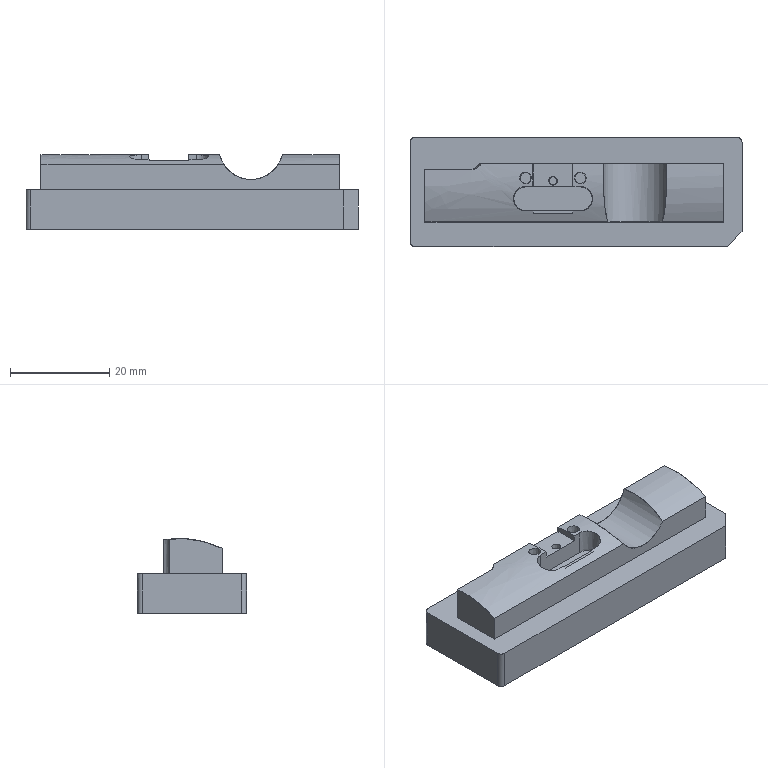NC program | PowerMill | posted with a generic post | part box 67 x 22 x 15.086 mm
Lines 17666 to 18440 of 221347:
N17763 M6
N17764 S22000 M03
N17765 G00 G90 X0.0 Y0.0
N17766 G43 Z9.7955 H27
N17767
N17768 G05 P10000 R4
N17769 X-4.5617 Y1.9439
N17770 Z-0.2426
N17771 G01 Z-1.4426 F1200.0
N17772 X-4.5093 Y1.9588 Z-1.4435
N17773 X-4.4875 Y1.965 Z-1.4439
N17774 X-4.3955 Y2.0345 Z-1.4459
N17775 X-4.3343 Y2.1329 Z-1.448
N17776 X-4.3126 Y2.2474 Z-1.45
N17777 X-4.3339 Y2.3611 Z-1.452
N17778 X-4.3945 Y2.4592 Z-1.454
N17779 X-4.441 Y2.4946 Z-1.4551
N17780 X-4.4875 Y2.5298 Z-1.4561
N17781 X-4.5983 Y2.5614 Z-1.4581
N17782 X-4.7137 Y2.5509 Z-1.4601
N17783 X-4.8179 Y2.4993 Z-1.4621
N17784 X-4.8959 Y2.4139 Z-1.4642
N17785 X-4.9382 Y2.3054 Z-1.4662
N17786 Y2.1897 Z-1.4682
N17787 X-4.8965 Y2.0817 Z-1.4702
N17788 X-4.8632 Y2.0451 Z-1.4711
N17789 X-4.8137 Y1.9937 Z-1.4723
N17790 X-4.7145 Y1.944 Z-1.4743
N17791 X-4.599 Y1.9333 Z-1.4763
N17792 X-4.5954 Y1.9343 Z-1.4764
N17793 X-4.5093 Y1.9588 Z-1.4779
N17794 X-4.4875 Y1.965 Z-1.4783
N17795 X-4.3955 Y2.0345 Z-1.4803
N17796 X-4.3343 Y2.1329 Z-1.4824
N17797 X-4.3126 Y2.2474 Z-1.4844
N17798 X-4.3339 Y2.3611 Z-1.4864
N17799 X-4.3945 Y2.4592 Z-1.4884
N17800 X-4.441 Y2.4946 Z-1.4894
N17801 X-4.4875 Y2.5298 Z-1.4905
N17802 X-4.5983 Y2.5614 Z-1.4925
N17803 X-4.7137 Y2.5509 Z-1.4945
N17804 X-4.8179 Y2.4993 Z-1.4965
N17805 X-4.8959 Y2.4139 Z-1.4985
N17806 X-4.9382 Y2.3054 Z-1.5006
N17807 Y2.1897 Z-1.5026
N17808 X-4.8965 Y2.0817 Z-1.5046
N17809 X-4.8632 Y2.0451 Z-1.5055
N17810 X-4.8137 Y1.9937 Z-1.5067
N17811 X-4.7145 Y1.944 Z-1.5087
N17812 X-4.599 Y1.9333 Z-1.5107
N17813 X-4.5954 Y1.9343
N17814 X-4.5093 Y1.9588 Z-1.5123
N17815 X-4.4875 Y1.965 Z-1.5127
N17816 X-4.3955 Y2.0345 Z-1.5147
N17817 X-4.3343 Y2.1329 Z-1.5167
N17818 X-4.3126 Y2.2474 Z-1.5188
N17819 X-4.3339 Y2.3611 Z-1.5208
N17820 X-4.3945 Y2.4592 Z-1.5228
N17821 X-4.441 Y2.4946 Z-1.5238
N17822 X-4.4875 Y2.5298 Z-1.5248
N17823 X-4.5983 Y2.5614 Z-1.5269
N17824 X-4.7137 Y2.5509 Z-1.5289
N17825 X-4.8179 Y2.4993 Z-1.5309
N17826 X-4.8959 Y2.4139 Z-1.5329
N17827 X-4.9382 Y2.3054 Z-1.535
N17828 Y2.1897 Z-1.537
N17829 X-4.8965 Y2.0817 Z-1.539
N17830 X-4.8632 Y2.0451 Z-1.5399
N17831 X-4.8137 Y1.9937 Z-1.5411
N17832 X-4.7145 Y1.944 Z-1.543
N17833 X-4.599 Y1.9333 Z-1.5451
N17834 X-4.5954 Y1.9343
N17835 X-4.5093 Y1.9588 Z-1.5467
N17836 X-4.4875 Y1.965 Z-1.5471
N17837 X-4.3955 Y2.0345 Z-1.5491
N17838 X-4.3343 Y2.1329 Z-1.5511
N17839 X-4.3126 Y2.2474 Z-1.5532
N17840 X-4.3339 Y2.3611 Z-1.5552
N17841 X-4.3945 Y2.4592 Z-1.5572
N17842 X-4.441 Y2.4946 Z-1.5582
N17843 X-4.4875 Y2.5298 Z-1.5592
N17844 X-4.5983 Y2.5614 Z-1.5612
N17845 X-4.7137 Y2.5509 Z-1.5633
N17846 X-4.8179 Y2.4993 Z-1.5653
N17847 X-4.8959 Y2.4139 Z-1.5673
N17848 X-4.9382 Y2.3054 Z-1.5693
N17849 Y2.1897 Z-1.5714
N17850 X-4.8965 Y2.0817 Z-1.5734
N17851 X-4.8632 Y2.0451 Z-1.5742
N17852 X-4.8137 Y1.9937 Z-1.5755
N17853 X-4.7145 Y1.944 Z-1.5774
N17854 X-4.599 Y1.9333 Z-1.5794
N17855 X-4.5954 Y1.9343 Z-1.5795
N17856 X-4.5093 Y1.9588 Z-1.5811
N17857 X-4.4875 Y1.965 Z-1.5815
N17858 X-4.3955 Y2.0345 Z-1.5835
N17859 X-4.3343 Y2.1329 Z-1.5855
N17860 X-4.3126 Y2.2474 Z-1.5875
N17861 X-4.3339 Y2.3611 Z-1.5896
N17862 X-4.3945 Y2.4592 Z-1.5916
N17863 X-4.441 Y2.4946 Z-1.5926
N17864 X-4.4229 Y2.5184
N17865 X-4.4739 Y2.5572 F2000.0
N17866 X-4.5955 Y2.5918
N17867 X-4.722 Y2.5803
N17868 X-4.8363 Y2.5237
N17869 X-4.9219 Y2.43
N17870 X-4.9682 Y2.311
N17871 Y2.1841
N17872 X-4.9224 Y2.0656
N17873 X-4.8851 Y2.0246
N17874 X-4.8317 Y1.9692
N17875 X-4.7229 Y1.9147
N17876 X-4.5962 Y1.9029
N17877 X-4.5872 Y1.9055
N17878 X-4.5011 Y1.93
N17879 X-4.4739 Y1.9377
N17880 X-4.3729 Y2.0139
N17881 X-4.3058 Y2.1218
N17882 X-4.2821 Y2.2473
N17883 X-4.3054 Y2.3722
N17884 X-4.3719 Y2.4797
N17885 X-4.4229 Y2.5184
N17886 X-4.5844 Y1.9385 Z-1.4919
N17887 X-4.5123 Y1.9588 Z-1.4932 F1200.0
N17888 X-4.488 Y1.9657 Z-1.4937
N17889 X-4.3961 Y2.0351 Z-1.4957
N17890 X-4.335 Y2.1333 Z-1.4977
N17891 X-4.3136 Y2.247 Z-1.4997
N17892 X-4.3347 Y2.3607 Z-1.5017
N17893 X-4.3951 Y2.4587 Z-1.5037
N17894 X-4.4415 Y2.4939 Z-1.5048
N17895 X-4.4873 Y2.5286 Z-1.5058
N17896 X-4.5989 Y2.5607 Z-1.5078
N17897 X-4.7137 Y2.5501 Z-1.5098
N17898 X-4.8174 Y2.4986 Z-1.5118
N17899 X-4.8954 Y2.4132 Z-1.5138
N17900 X-4.9372 Y2.3056 Z-1.5159
N17901 X-4.9374 Y2.1904 Z-1.5179
N17902 X-4.8959 Y2.0826 Z-1.5199
N17903 X-4.84 Y2.021 Z-1.5213
N17904 X-4.815 Y1.995 Z-1.522
N17905 X-4.7147 Y1.9451 Z-1.5239
N17906 X-4.5996 Y1.9342 Z-1.5259
N17907 X-4.596 Y1.9352 Z-1.526
N17908 X-4.5123 Y1.9588 Z-1.5275
N17909 X-4.488 Y1.9657 Z-1.528
N17910 X-4.3961 Y2.0351 Z-1.53
N17911 X-4.335 Y2.1333 Z-1.532
N17912 X-4.3136 Y2.247 Z-1.534
N17913 X-4.3347 Y2.3607 Z-1.536
N17914 X-4.3951 Y2.4587 Z-1.538
N17915 X-4.4415 Y2.4939 Z-1.539
N17916 X-4.4873 Y2.5286 Z-1.5401
N17917 X-4.5989 Y2.5607 Z-1.5421
N17918 X-4.7137 Y2.5501 Z-1.5441
N17919 X-4.8174 Y2.4986 Z-1.5461
N17920 X-4.8954 Y2.4132 Z-1.5481
N17921 X-4.9372 Y2.3056 Z-1.5501
N17922 X-4.9374 Y2.1904 Z-1.5522
N17923 X-4.8959 Y2.0826 Z-1.5542
N17924 X-4.84 Y2.021 Z-1.5556
N17925 X-4.815 Y1.995 Z-1.5563
N17926 X-4.7147 Y1.9451 Z-1.5582
N17927 X-4.5996 Y1.9342 Z-1.5602
N17928 X-4.596 Y1.9352 Z-1.5603
N17929 X-4.5123 Y1.9588 Z-1.5618
N17930 X-4.488 Y1.9657 Z-1.5622
N17931 X-4.3961 Y2.0351 Z-1.5643
N17932 X-4.335 Y2.1333 Z-1.5663
N17933 X-4.3136 Y2.247 Z-1.5683
N17934 X-4.3347 Y2.3607 Z-1.5703
N17935 X-4.3951 Y2.4587 Z-1.5723
N17936 X-4.4415 Y2.4939 Z-1.5733
N17937 X-4.4873 Y2.5286 Z-1.5743
N17938 X-4.5989 Y2.5607 Z-1.5764
N17939 X-4.7137 Y2.5501 Z-1.5784
N17940 X-4.8174 Y2.4986 Z-1.5804
N17941 X-4.8954 Y2.4132 Z-1.5824
N17942 X-4.9372 Y2.3056 Z-1.5844
N17943 X-4.9374 Y2.1904 Z-1.5864
N17944 X-4.8959 Y2.0826 Z-1.5885
N17945 X-4.84 Y2.021 Z-1.5899
N17946 X-4.815 Y1.995 Z-1.5905
N17947 X-4.7147 Y1.9451 Z-1.5925
N17948 X-4.5996 Y1.9342 Z-1.5945
N17949 X-4.596 Y1.9352 Z-1.5946
N17950 X-4.5123 Y1.9588 Z-1.5961
N17951 X-4.488 Y1.9657 Z-1.5965
N17952 X-4.3961 Y2.0351 Z-1.5985
N17953 X-4.335 Y2.1333 Z-1.6006
N17954 X-4.3136 Y2.247 Z-1.6026
N17955 X-4.3347 Y2.3607 Z-1.6046
N17956 X-4.3951 Y2.4587 Z-1.6066
N17957 X-4.4415 Y2.4939 Z-1.6076
N17958 X-4.4873 Y2.5286 Z-1.6086
N17959 X-4.5989 Y2.5607 Z-1.6107
N17960 X-4.7137 Y2.5501 Z-1.6127
N17961 X-4.8174 Y2.4986 Z-1.6147
N17962 X-4.8954 Y2.4132 Z-1.6167
N17963 X-4.9372 Y2.3056 Z-1.6187
N17964 X-4.9374 Y2.1904 Z-1.6207
N17965 X-4.8959 Y2.0826 Z-1.6228
N17966 X-4.84 Y2.021 Z-1.6242
N17967 X-4.815 Y1.995 Z-1.6248
N17968 X-4.7147 Y1.9451 Z-1.6268
N17969 X-4.5996 Y1.9342 Z-1.6288
N17970 X-4.596 Y1.9352 Z-1.6289
N17971 X-4.5123 Y1.9588 Z-1.6304
N17972 X-4.488 Y1.9657 Z-1.6308
N17973 X-4.3961 Y2.0351 Z-1.6328
N17974 X-4.335 Y2.1333 Z-1.6349
N17975 X-4.3136 Y2.247 Z-1.6369
N17976 X-4.3347 Y2.3607 Z-1.6389
N17977 X-4.3951 Y2.4587 Z-1.6409
N17978 X-4.4415 Y2.4939 Z-1.6419
N17979 X-4.4234 Y2.5178
N17980 X-4.4736 Y2.5559 F2000.0
N17981 X-4.596 Y2.591
N17982 X-4.722 Y2.5794
N17983 X-4.8358 Y2.523
N17984 X-4.9214 Y2.4293
N17985 X-4.9672 Y2.3112
N17986 X-4.9674 Y2.1849
N17987 X-4.9219 Y2.0666
N17988 X-4.8619 Y2.0005
N17989 X-4.833 Y1.9705
N17990 X-4.7231 Y1.9157
N17991 X-4.5968 Y1.9038
N17992 X-4.5878 Y1.9063
N17993 X-4.5041 Y1.93
N17994 X-4.4744 Y1.9384
N17995 X-4.3736 Y2.0145
N17996 X-4.3066 Y2.1223
N17997 X-4.283 Y2.247
N17998 X-4.3062 Y2.3717
N17999 X-4.3726 Y2.4792
N18000 X-4.4234 Y2.5178
N18001 X-4.6067 Y1.9357 Z-1.5412
N18002 X-4.5996 Y1.935 Z-1.5414 F1200.0
N18003 X-4.596 Y1.936
N18004 X-4.5154 Y1.9588 Z-1.5429
N18005 X-4.4889 Y1.9664 Z-1.5434
N18006 X-4.3968 Y2.0356 Z-1.5454
N18007 X-4.3359 Y2.1335 Z-1.5474
N18008 X-4.3144 Y2.2473 Z-1.5494
N18009 X-4.3354 Y2.36 Z-1.5514
N18010 X-4.3962 Y2.4588 Z-1.5535
N18011 X-4.4419 Y2.4933 Z-1.5545
N18012 X-4.4876 Y2.5278 Z-1.5555
N18013 X-4.5988 Y2.5597 Z-1.5575
N18014 X-4.7132 Y2.5493 Z-1.5595
N18015 X-4.8172 Y2.4978 Z-1.5615
N18016 X-4.8948 Y2.4127 Z-1.5635
N18017 X-4.9364 Y2.3055 Z-1.5655
N18018 X-4.9365 Y2.1903 Z-1.5675
N18019 X-4.8951 Y2.0829 Z-1.5695
N18020 X-4.8198 Y1.9999 Z-1.5715
N18021 X-4.8171 Y1.9971 Z-1.5716
N18022 X-4.714 Y1.9457 Z-1.5736
N18023 X-4.5996 Y1.935 Z-1.5756
N18024 X-4.596 Y1.936
N18025 X-4.5154 Y1.9588 Z-1.5771
N18026 X-4.4889 Y1.9664 Z-1.5776
N18027 X-4.3968 Y2.0356 Z-1.5796
N18028 X-4.3359 Y2.1335 Z-1.5816
N18029 X-4.3144 Y2.2473 Z-1.5836
N18030 X-4.3354 Y2.36 Z-1.5856
N18031 X-4.3962 Y2.4588 Z-1.5877
N18032 X-4.4419 Y2.4933 Z-1.5887
N18033 X-4.4876 Y2.5278 Z-1.5897
N18034 X-4.5988 Y2.5597 Z-1.5917
N18035 X-4.7132 Y2.5493 Z-1.5937
N18036 X-4.8172 Y2.4978 Z-1.5957
N18037 X-4.8948 Y2.4127 Z-1.5977
N18038 X-4.9364 Y2.3055 Z-1.5997
N18039 X-4.9365 Y2.1903 Z-1.6017
N18040 X-4.8951 Y2.0829 Z-1.6037
N18041 X-4.8198 Y1.9999 Z-1.6057
N18042 X-4.8171 Y1.9971 Z-1.6058
N18043 X-4.714 Y1.9457 Z-1.6078
N18044 X-4.5996 Y1.935 Z-1.6098
N18045 X-4.596 Y1.936
N18046 X-4.5154 Y1.9588 Z-1.6113
N18047 X-4.4889 Y1.9664 Z-1.6118
N18048 X-4.3968 Y2.0356 Z-1.6138
N18049 X-4.3359 Y2.1335 Z-1.6158
N18050 X-4.3144 Y2.2473 Z-1.6178
N18051 X-4.3354 Y2.36 Z-1.6198
N18052 X-4.3962 Y2.4588 Z-1.6219
N18053 X-4.4419 Y2.4933 Z-1.6229
N18054 X-4.4876 Y2.5278 Z-1.6239
N18055 X-4.5988 Y2.5597 Z-1.6259
N18056 X-4.7132 Y2.5493 Z-1.6279
N18057 X-4.8172 Y2.4978 Z-1.6299
N18058 X-4.8948 Y2.4127 Z-1.6319
N18059 X-4.9364 Y2.3055 Z-1.6339
N18060 X-4.9365 Y2.1903 Z-1.6359
N18061 X-4.8951 Y2.0829 Z-1.6379
N18062 X-4.8198 Y1.9999 Z-1.6399
N18063 X-4.8171 Y1.9971 Z-1.64
N18064 X-4.714 Y1.9457 Z-1.642
N18065 X-4.5996 Y1.935 Z-1.644
N18066 X-4.596 Y1.936
N18067 X-4.5154 Y1.9588 Z-1.6455
N18068 X-4.4889 Y1.9664 Z-1.646
N18069 X-4.3968 Y2.0356 Z-1.648
N18070 X-4.3359 Y2.1335 Z-1.65
N18071 X-4.3144 Y2.2473 Z-1.652
N18072 X-4.3354 Y2.36 Z-1.654
N18073 X-4.3962 Y2.4588 Z-1.6561
N18074 X-4.4419 Y2.4933 Z-1.6571
N18075 X-4.4876 Y2.5278 Z-1.6581
N18076 X-4.5988 Y2.5597 Z-1.6601
N18077 X-4.7132 Y2.5493 Z-1.6621
N18078 X-4.8172 Y2.4978 Z-1.6641
N18079 X-4.8948 Y2.4127 Z-1.6661
N18080 X-4.9364 Y2.3055 Z-1.6681
N18081 X-4.9365 Y2.1903 Z-1.6701
N18082 X-4.8951 Y2.0829 Z-1.6721
N18083 X-4.8198 Y1.9999 Z-1.6741
N18084 X-4.8171 Y1.9971 Z-1.6742
N18085 X-4.714 Y1.9457 Z-1.6762
N18086 X-4.5996 Y1.935 Z-1.6782
N18087 X-4.596 Y1.936
N18088 X-4.5154 Y1.9588 Z-1.6797
N18089 X-4.4889 Y1.9664 Z-1.6802
N18090 X-4.3968 Y2.0356 Z-1.6822
N18091 X-4.3359 Y2.1335 Z-1.6842
N18092 X-4.3144 Y2.2473 Z-1.6862
N18093 X-4.3354 Y2.36 Z-1.6882
N18094 X-4.3962 Y2.4588 Z-1.6903
N18095 X-4.4419 Y2.4933 Z-1.6912
N18096 X-4.4238 Y2.5172
N18097 X-4.474 Y2.5551 F2000.0
N18098 X-4.5959 Y2.5901
N18099 X-4.7215 Y2.5786
N18100 X-4.8355 Y2.5222
N18101 X-4.9207 Y2.4288
N18102 X-4.9663 Y2.3112
N18103 X-4.9665 Y2.1847
N18104 X-4.9211 Y2.0669
N18105 X-4.8417 Y1.9795
N18106 X-4.8351 Y1.9726
N18107 X-4.7224 Y1.9163
N18108 X-4.5968 Y1.9046
N18109 X-4.5879 Y1.9072
N18110 X-4.5072 Y1.93
N18111 X-4.4753 Y1.939
N18112 X-4.3743 Y2.015
N18113 X-4.3075 Y2.1224
N18114 X-4.2839 Y2.2472
N18115 X-4.3069 Y2.371
N18116 X-4.3736 Y2.4793
N18117 X-4.4238 Y2.5172
N18118 X-4.6301 Y1.9387 Z-1.5906
N18119 X-4.5996 Y1.9359 Z-1.5911 F1200.0
N18120 X-4.596 Y1.9369 Z-1.5912
N18121 X-4.5185 Y1.9588 Z-1.5926
N18122 X-4.4889 Y1.9672 Z-1.5931
N18123 X-4.3972 Y2.0364 Z-1.5951
N18124 X-4.3365 Y2.1341 Z-1.5971
N18125 X-4.3153 Y2.2471 Z-1.5991
N18126 X-4.3362 Y2.3599 Z-1.6011
N18127 X-4.3966 Y2.4578 Z-1.6031
N18128 X-4.4425 Y2.4926 Z-1.6041
N18129 X-4.4879 Y2.527 Z-1.6051
N18130 X-4.5986 Y2.5588 Z-1.6072
N18131 X-4.7129 Y2.5485 Z-1.6092
N18132 X-4.8163 Y2.4973 Z-1.6112
N18133 X-4.894 Y2.4124 Z-1.6132
N18134 X-4.9356 Y2.3051 Z-1.6152
N18135 X-4.9357 Y2.1901 Z-1.6172
N18136 X-4.8945 Y2.0836 Z-1.6192
N18137 X-4.8171 Y1.9982 Z-1.6212
N18138 X-4.7139 Y1.9466 Z-1.6232
N18139 X-4.5996 Y1.9359 Z-1.6252
N18140 X-4.596 Y1.9369 Z-1.6253
N18141 X-4.5185 Y1.9588 Z-1.6267
N18142 X-4.4889 Y1.9672 Z-1.6272
N18143 X-4.3972 Y2.0364 Z-1.6292
N18144 X-4.3365 Y2.1341 Z-1.6312
N18145 X-4.3153 Y2.2471 Z-1.6332
N18146 X-4.3362 Y2.3599 Z-1.6352
N18147 X-4.3966 Y2.4578 Z-1.6372
N18148 X-4.4425 Y2.4926 Z-1.6383
N18149 X-4.4879 Y2.527 Z-1.6392
N18150 X-4.5986 Y2.5588 Z-1.6413
N18151 X-4.7129 Y2.5485 Z-1.6433
N18152 X-4.8163 Y2.4973 Z-1.6453
N18153 X-4.894 Y2.4124 Z-1.6473
N18154 X-4.9356 Y2.3051 Z-1.6493
N18155 X-4.9357 Y2.1901 Z-1.6513
N18156 X-4.8945 Y2.0836 Z-1.6533
N18157 X-4.8171 Y1.9982 Z-1.6553
N18158 X-4.7139 Y1.9466 Z-1.6573
N18159 X-4.5996 Y1.9359 Z-1.6593
N18160 X-4.596 Y1.9369 Z-1.6594
N18161 X-4.5185 Y1.9588 Z-1.6608
N18162 X-4.4889 Y1.9672 Z-1.6613
N18163 X-4.3972 Y2.0364 Z-1.6633
N18164 X-4.3365 Y2.1341 Z-1.6653
N18165 X-4.3153 Y2.2471 Z-1.6673
N18166 X-4.3362 Y2.3599 Z-1.6693
N18167 X-4.3966 Y2.4578 Z-1.6714
N18168 X-4.4425 Y2.4926 Z-1.6724
N18169 X-4.4879 Y2.527 Z-1.6734
N18170 X-4.5986 Y2.5588 Z-1.6754
N18171 X-4.7129 Y2.5485 Z-1.6774
N18172 X-4.8163 Y2.4973 Z-1.6794
N18173 X-4.894 Y2.4124 Z-1.6814
N18174 X-4.9356 Y2.3051 Z-1.6834
N18175 X-4.9357 Y2.1901 Z-1.6854
N18176 X-4.8945 Y2.0836 Z-1.6874
N18177 X-4.8171 Y1.9982 Z-1.6894
N18178 X-4.7139 Y1.9466 Z-1.6914
N18179 X-4.5996 Y1.9359 Z-1.6934
N18180 X-4.596 Y1.9369 Z-1.6935
N18181 X-4.5185 Y1.9588 Z-1.6949
N18182 X-4.4889 Y1.9672 Z-1.6954
N18183 X-4.3972 Y2.0364 Z-1.6974
N18184 X-4.3365 Y2.1341 Z-1.6994
N18185 X-4.3153 Y2.2471 Z-1.7014
N18186 X-4.3362 Y2.3599 Z-1.7035
N18187 X-4.3966 Y2.4578 Z-1.7055
N18188 X-4.4425 Y2.4926 Z-1.7065
N18189 X-4.4879 Y2.527 Z-1.7075
N18190 X-4.5986 Y2.5588 Z-1.7095
N18191 X-4.7129 Y2.5485 Z-1.7115
N18192 X-4.8163 Y2.4973 Z-1.7135
N18193 X-4.894 Y2.4124 Z-1.7155
N18194 X-4.9356 Y2.3051 Z-1.7175
N18195 X-4.9357 Y2.1901 Z-1.7195
N18196 X-4.8945 Y2.0836 Z-1.7215
N18197 X-4.8171 Y1.9982 Z-1.7235
N18198 X-4.7139 Y1.9466 Z-1.7255
N18199 X-4.5996 Y1.9359 Z-1.7275
N18200 X-4.596 Y1.9369 Z-1.7276
N18201 X-4.5185 Y1.9588 Z-1.729
N18202 X-4.4889 Y1.9672 Z-1.7295
N18203 X-4.3972 Y2.0364 Z-1.7315
N18204 X-4.3365 Y2.1341 Z-1.7335
N18205 X-4.3153 Y2.2471 Z-1.7356
N18206 X-4.3362 Y2.3599 Z-1.7376
N18207 X-4.3966 Y2.4578 Z-1.7396
N18208 X-4.4425 Y2.4926 Z-1.7406
N18209 X-4.4244 Y2.5165
N18210 X-4.4743 Y2.5543 F2000.0
N18211 X-4.5957 Y2.5892
N18212 X-4.7212 Y2.5778
N18213 X-4.8346 Y2.5217
N18214 X-4.9199 Y2.4284
N18215 X-4.9656 Y2.3107
N18216 X-4.9657 Y2.1845
N18217 X-4.9204 Y2.0675
N18218 X-4.8356 Y1.9739
N18219 X-4.7223 Y1.9172
N18220 X-4.5968 Y1.9055
N18221 X-4.5879 Y1.908
N18222 X-4.5103 Y1.93
N18223 X-4.4754 Y1.9399
N18224 X-4.3746 Y2.0158
N18225 X-4.3081 Y2.123
N18226 X-4.2847 Y2.247
N18227 X-4.3078 Y2.3709
N18228 X-4.374 Y2.4784
N18229 X-4.4244 Y2.5165
N18230 X-4.6814 Y1.9444 Z-1.6399
N18231 X-4.5996 Y1.9367 Z-1.6413 F1200.0
N18232 X-4.5216 Y1.9588 Z-1.6427
N18233 X-4.4897 Y1.9679 Z-1.6433
N18234 X-4.4044 Y2.032 Z-1.6452
N18235 X-4.3978 Y2.0408 Z-1.6454
N18236 X-4.3188 Y2.2442 Z-1.6492
N18237 X-4.3178 Y2.2551 Z-1.6494
N18238 X-4.337 Y2.3596 Z-1.6512
N18239 X-4.3971 Y2.457 Z-1.6532
N18240 X-4.443 Y2.4919 Z-1.6542
N18241 X-4.4883 Y2.5262 Z-1.6552
N18242 X-4.5993 Y2.5581 Z-1.6572
N18243 X-4.7132 Y2.5476 Z-1.6592
N18244 X-4.8157 Y2.4967 Z-1.6612
N18245 X-4.8934 Y2.4117 Z-1.6632
N18246 X-4.9346 Y2.3053 Z-1.6652
N18247 X-4.9348 Y2.1906 Z-1.6672
N18248 X-4.8935 Y2.0835 Z-1.6692
N18249 X-4.8163 Y1.9986 Z-1.6712
N18250 X-4.7137 Y1.9474 Z-1.6732
N18251 X-4.5996 Y1.9367 Z-1.6752
N18252 X-4.5216 Y1.9588 Z-1.6767
N18253 X-4.4897 Y1.9679 Z-1.6772
N18254 X-4.4044 Y2.032 Z-1.6791
N18255 X-4.3978 Y2.0408 Z-1.6793
N18256 X-4.3188 Y2.2442 Z-1.6831
N18257 X-4.3178 Y2.2551 Z-1.6833
N18258 X-4.337 Y2.3596 Z-1.6852
N18259 X-4.3971 Y2.457 Z-1.6871
N18260 X-4.443 Y2.4919 Z-1.6882
N18261 X-4.4883 Y2.5262 Z-1.6891
N18262 X-4.5993 Y2.5581 Z-1.6912
N18263 X-4.7132 Y2.5476 Z-1.6932
N18264 X-4.8157 Y2.4967 Z-1.6952
N18265 X-4.8934 Y2.4117 Z-1.6972
N18266 X-4.9346 Y2.3053 Z-1.6992
N18267 X-4.9348 Y2.1906 Z-1.7012
N18268 X-4.8935 Y2.0835 Z-1.7032
N18269 X-4.8163 Y1.9986 Z-1.7052
N18270 X-4.7137 Y1.9474 Z-1.7072
N18271 X-4.5996 Y1.9367 Z-1.7092
N18272 X-4.5216 Y1.9588 Z-1.7106
N18273 X-4.4897 Y1.9679 Z-1.7112
N18274 X-4.4044 Y2.032 Z-1.713
N18275 X-4.3978 Y2.0408 Z-1.7132
N18276 X-4.3188 Y2.2442 Z-1.717
N18277 X-4.3178 Y2.2551 Z-1.7172
N18278 X-4.337 Y2.3596 Z-1.7191
N18279 X-4.3971 Y2.457 Z-1.7211
N18280 X-4.443 Y2.4919 Z-1.7221
N18281 X-4.4883 Y2.5262 Z-1.7231
N18282 X-4.5993 Y2.5581 Z-1.7251
N18283 X-4.7132 Y2.5476 Z-1.7271
N18284 X-4.8157 Y2.4967 Z-1.7291
N18285 X-4.8934 Y2.4117 Z-1.7311
N18286 X-4.9346 Y2.3053 Z-1.7331
N18287 X-4.9348 Y2.1906 Z-1.7351
N18288 X-4.8935 Y2.0835 Z-1.7371
N18289 X-4.8163 Y1.9986 Z-1.7391
N18290 X-4.7137 Y1.9474 Z-1.7411
N18291 X-4.5996 Y1.9367 Z-1.7431
N18292 X-4.5216 Y1.9588 Z-1.7445
N18293 X-4.4897 Y1.9679 Z-1.7451
N18294 X-4.4044 Y2.032 Z-1.7469
N18295 X-4.3978 Y2.0408 Z-1.7471
N18296 X-4.3188 Y2.2442 Z-1.7509
N18297 X-4.3178 Y2.2551 Z-1.7511
N18298 X-4.337 Y2.3596 Z-1.753
N18299 X-4.3971 Y2.457 Z-1.755
N18300 X-4.443 Y2.4919 Z-1.756
N18301 X-4.4883 Y2.5262 Z-1.757
N18302 X-4.5993 Y2.5581 Z-1.759
N18303 X-4.7132 Y2.5476 Z-1.761
N18304 X-4.8157 Y2.4967 Z-1.763
N18305 X-4.8934 Y2.4117 Z-1.765
N18306 X-4.9346 Y2.3053 Z-1.767
N18307 X-4.9348 Y2.1906 Z-1.769
N18308 X-4.8935 Y2.0835 Z-1.771
N18309 X-4.8163 Y1.9986 Z-1.773
N18310 X-4.7137 Y1.9474 Z-1.775
N18311 X-4.5996 Y1.9367 Z-1.777
N18312 X-4.5216 Y1.9588 Z-1.7784
N18313 X-4.4897 Y1.9679 Z-1.779
N18314 X-4.4044 Y2.032 Z-1.7809
N18315 X-4.3978 Y2.0408 Z-1.781
N18316 X-4.3188 Y2.2442 Z-1.7849
N18317 X-4.3178 Y2.2551 Z-1.785
N18318 X-4.337 Y2.3596 Z-1.7869
N18319 X-4.3971 Y2.457 Z-1.7889
N18320 X-4.443 Y2.4919 Z-1.7899
N18321 X-4.4249 Y2.5158
N18322 X-4.4747 Y2.5535 F2000.0
N18323 X-4.5964 Y2.5885
N18324 X-4.7216 Y2.5769
N18325 X-4.834 Y2.5211
N18326 X-4.9193 Y2.4278
N18327 X-4.9646 Y2.3109
N18328 X-4.9648 Y2.1851
N18329 X-4.9195 Y2.0675
N18330 X-4.8347 Y1.9743
N18331 X-4.7221 Y1.9181
N18332 X-4.5968 Y1.9064
N18333 X-4.5134 Y1.93
N18334 X-4.4761 Y1.9406
N18335 X-4.3864 Y2.0081
N18336 X-4.3766 Y2.0178
N18337 X-4.3698 Y2.0299
N18338 X-4.2908 Y2.2334
N18339 X-4.2877 Y2.2468
N18340 X-4.2883 Y2.2606
N18341 X-4.3086 Y2.3706
N18342 X-4.3745 Y2.4775
N18343 X-4.4249 Y2.5158
N18344 X-4.7051 Y1.9474 Z-1.6892
N18345 X-4.5996 Y1.9376 Z-1.6911 F1200.0
N18346 X-4.5247 Y1.9588 Z-1.6924
N18347 X-4.4896 Y1.9688 Z-1.6931
N18348 X-4.4054 Y2.0323 Z-1.6949
N18349 X-4.3988 Y2.041 Z-1.6951
N18350 X-4.3196 Y2.2448 Z-1.6989
N18351 X-4.3185 Y2.2557 Z-1.6991
N18352 X-4.3378 Y2.3593 Z-1.7009
N18353 X-4.3977 Y2.4563 Z-1.7029
N18354 X-4.4436 Y2.4912 Z-1.7039
N18355 X-4.4889 Y2.5256 Z-1.7049
N18356 X-4.5991 Y2.5572 Z-1.7069
N18357 X-4.7124 Y2.5468 Z-1.7089
N18358 X-4.8156 Y2.4958 Z-1.7109
N18359 X-4.8924 Y2.4116 Z-1.7129
N18360 X-4.9337 Y2.3053 Z-1.7149
N18361 X-4.934 Y2.1904 Z-1.7169
N18362 X-4.8928 Y2.0838 Z-1.7189
N18363 X-4.8161 Y1.9996 Z-1.7209
N18364 X-4.7134 Y1.9482 Z-1.7229
N18365 X-4.5996 Y1.9376 Z-1.7249
N18366 X-4.5247 Y1.9588 Z-1.7262
N18367 X-4.4896 Y1.9688 Z-1.7269
N18368 X-4.4054 Y2.0323 Z-1.7287
N18369 X-4.3988 Y2.041 Z-1.7289
N18370 X-4.3196 Y2.2448 Z-1.7327
N18371 X-4.3185 Y2.2557 Z-1.7329
N18372 X-4.3378 Y2.3593 Z-1.7348
N18373 X-4.3977 Y2.4563 Z-1.7368
N18374 X-4.4436 Y2.4912 Z-1.7378
N18375 X-4.4889 Y2.5256 Z-1.7388
N18376 X-4.5991 Y2.5572 Z-1.7408
N18377 X-4.7124 Y2.5468 Z-1.7427
N18378 X-4.8156 Y2.4958 Z-1.7447
N18379 X-4.8924 Y2.4116 Z-1.7467
N18380 X-4.9337 Y2.3053 Z-1.7487
N18381 X-4.934 Y2.1904 Z-1.7507
N18382 X-4.8928 Y2.0838 Z-1.7527
N18383 X-4.8161 Y1.9996 Z-1.7547
N18384 X-4.7134 Y1.9482 Z-1.7567
N18385 X-4.5996 Y1.9376 Z-1.7587
N18386 X-4.5247 Y1.9588 Z-1.7601
N18387 X-4.4896 Y1.9688 Z-1.7607
N18388 X-4.4054 Y2.0323 Z-1.7625
N18389 X-4.3988 Y2.041 Z-1.7627
N18390 X-4.3196 Y2.2448 Z-1.7666
N18391 X-4.3185 Y2.2557 Z-1.7667
N18392 X-4.3378 Y2.3593 Z-1.7686
N18393 X-4.3977 Y2.4563 Z-1.7706
N18394 X-4.4436 Y2.4912 Z-1.7716
N18395 X-4.4889 Y2.5256 Z-1.7726
N18396 X-4.5991 Y2.5572 Z-1.7746
N18397 X-4.7124 Y2.5468 Z-1.7766
N18398 X-4.8156 Y2.4958 Z-1.7786
N18399 X-4.8924 Y2.4116 Z-1.7806
N18400 X-4.9337 Y2.3053 Z-1.7825
N18401 X-4.934 Y2.1904 Z-1.7846
N18402 X-4.8928 Y2.0838 Z-1.7865
N18403 X-4.8161 Y1.9996 Z-1.7885
N18404 X-4.7134 Y1.9482 Z-1.7905
N18405 X-4.5996 Y1.9376 Z-1.7925
N18406 X-4.5247 Y1.9588 Z-1.7939
N18407 X-4.4896 Y1.9688 Z-1.7945
N18408 X-4.4054 Y2.0323 Z-1.7964
N18409 X-4.3988 Y2.041 Z-1.7966
N18410 X-4.3196 Y2.2448 Z-1.8004
N18411 X-4.3185 Y2.2557 Z-1.8006
N18412 X-4.3378 Y2.3593 Z-1.8024
N18413 X-4.3977 Y2.4563 Z-1.8044
N18414 X-4.4436 Y2.4912 Z-1.8054
N18415 X-4.4889 Y2.5256 Z-1.8064
N18416 X-4.5991 Y2.5572 Z-1.8084
N18417 X-4.7124 Y2.5468 Z-1.8104
N18418 X-4.8156 Y2.4958 Z-1.8124
N18419 X-4.8924 Y2.4116 Z-1.8144
N18420 X-4.9337 Y2.3053 Z-1.8164
N18421 X-4.934 Y2.1904 Z-1.8184
N18422 X-4.8928 Y2.0838 Z-1.8204
N18423 X-4.8161 Y1.9996 Z-1.8224
N18424 X-4.7134 Y1.9482 Z-1.8244
N18425 X-4.5996 Y1.9376 Z-1.8264
N18426 X-4.5247 Y1.9588 Z-1.8277
N18427 X-4.4896 Y1.9688 Z-1.8283
N18428 X-4.4054 Y2.0323 Z-1.8302
N18429 X-4.3988 Y2.041 Z-1.8304
N18430 X-4.3196 Y2.2448 Z-1.8342
N18431 X-4.3185 Y2.2557 Z-1.8344
N18432 X-4.3378 Y2.3593 Z-1.8362
N18433 X-4.3977 Y2.4563 Z-1.8382
N18434 X-4.4436 Y2.4912 Z-1.8392
N18435 X-4.4254 Y2.5151
N18436 X-4.4753 Y2.5529 F2000.0
N18437 X-4.5963 Y2.5876
N18438 X-4.7207 Y2.5762
N18439 X-4.834 Y2.5201
N18440 X-4.9183 Y2.4277
N18441 X-4.9637 Y2.311
N18442 X-4.964 Y2.1849
N18443 X-4.9187 Y2.0678
N18444 X-4.8346 Y1.9753
N18445 X-4.7218 Y1.9189
N18446 X-4.5968 Y1.9072
N18447 X-4.5165 Y1.93
N18448 X-4.476 Y1.9415
N18449 X-4.3874 Y2.0083
N18450 X-4.3776 Y2.0181
N18451 X-4.3709 Y2.0301
N18452 X-4.2916 Y2.2339
N18453 X-4.2884 Y2.2474
N18454 X-4.2891 Y2.2612
N18455 X-4.3094 Y2.3703
N18456 X-4.3751 Y2.4768
N18457 X-4.4254 Y2.5151
N18458 X-4.7266 Y1.9557 Z-1.7386
N18459 X-4.7131 Y1.949 Z-1.7388 F1200.0
N18460 X-4.5995 Y1.9384 Z-1.7408
N18461 X-4.5278 Y1.9588 Z-1.7421
N18462 X-4.4902 Y1.9695 Z-1.7428
N18463 X-4.4058 Y2.0331 Z-1.7446
N18464 X-4.3992 Y2.0418 Z-1.7448
N18465 X-4.3205 Y2.2444 Z-1.7486
N18466 X-4.3195 Y2.2553 Z-1.7488
N18467 X-4.3387 Y2.359 Z-1.7506
N18468 X-4.3983 Y2.4558 Z-1.7526
N18469 X-4.4441 Y2.4905 Z-1.7536
N18470 X-4.4898 Y2.5252 Z-1.7546
N18471 X-4.599 Y2.5563 Z-1.7566
N18472 X-4.7125 Y2.5459 Z-1.7586
N18473 X-4.815 Y2.4951 Z-1.7606
N18474 X-4.8918 Y2.411 Z-1.7626
N18475 X-4.9328 Y2.3053 Z-1.7646
N18476 X-4.9331 Y2.1904 Z-1.7666
N18477 X-4.8921 Y2.0844 Z-1.7686
N18478 X-4.8154 Y2.0001 Z-1.7705
N18479 X-4.7131 Y1.949 Z-1.7725
N18480 X-4.5995 Y1.9384 Z-1.7745
N18481 X-4.5278 Y1.9588 Z-1.7758
N18482 X-4.4902 Y1.9695 Z-1.7765
N18483 X-4.4058 Y2.0331 Z-1.7784
N18484 X-4.3992 Y2.0418 Z-1.7786
N18485 X-4.3205 Y2.2444 Z-1.7823
N18486 X-4.3195 Y2.2553 Z-1.7825
N18487 X-4.3387 Y2.359 Z-1.7844
N18488 X-4.3983 Y2.4558 Z-1.7864
N18489 X-4.4441 Y2.4905 Z-1.7874
N18490 X-4.4898 Y2.5252 Z-1.7884
N18491 X-4.599 Y2.5563 Z-1.7903
N18492 X-4.7125 Y2.5459 Z-1.7923
N18493 X-4.815 Y2.4951 Z-1.7943
N18494 X-4.8918 Y2.411 Z-1.7963
N18495 X-4.9328 Y2.3053 Z-1.7983
N18496 X-4.9331 Y2.1904 Z-1.8003
N18497 X-4.8921 Y2.0844 Z-1.8023
N18498 X-4.8154 Y2.0001 Z-1.8043
N18499 X-4.7131 Y1.949 Z-1.8063
N18500 X-4.5995 Y1.9384 Z-1.8083
N18501 X-4.5278 Y1.9588 Z-1.8096
N18502 X-4.4902 Y1.9695 Z-1.8102
N18503 X-4.4058 Y2.0331 Z-1.8121
N18504 X-4.3992 Y2.0418 Z-1.8123
N18505 X-4.3205 Y2.2444 Z-1.8161
N18506 X-4.3195 Y2.2553 Z-1.8163
N18507 X-4.3387 Y2.359 Z-1.8181
N18508 X-4.3983 Y2.4558 Z-1.8201
N18509 X-4.4441 Y2.4905 Z-1.8211
N18510 X-4.4898 Y2.5252 Z-1.8221
N18511 X-4.599 Y2.5563 Z-1.8241
N18512 X-4.7125 Y2.5459 Z-1.8261
N18513 X-4.815 Y2.4951 Z-1.8281
N18514 X-4.8918 Y2.411 Z-1.83
N18515 X-4.9328 Y2.3053 Z-1.832
N18516 X-4.9331 Y2.1904 Z-1.834
N18517 X-4.8921 Y2.0844 Z-1.836
N18518 X-4.8154 Y2.0001 Z-1.838
N18519 X-4.7131 Y1.949 Z-1.84
N18520 X-4.5995 Y1.9384 Z-1.842
N18521 X-4.5278 Y1.9588 Z-1.8433
N18522 X-4.4902 Y1.9695 Z-1.844
N18523 X-4.4058 Y2.0331 Z-1.8458
N18524 X-4.3992 Y2.0418 Z-1.846
N18525 X-4.3205 Y2.2444 Z-1.8498
N18526 X-4.3195 Y2.2553 Z-1.85
N18527 X-4.3387 Y2.359 Z-1.8518
N18528 X-4.3983 Y2.4558 Z-1.8538
N18529 X-4.4441 Y2.4905 Z-1.8548
N18530 X-4.4898 Y2.5252 Z-1.8558
N18531 X-4.599 Y2.5563 Z-1.8578
N18532 X-4.7125 Y2.5459 Z-1.8598
N18533 X-4.815 Y2.4951 Z-1.8618
N18534 X-4.8918 Y2.411 Z-1.8638
N18535 X-4.9328 Y2.3053 Z-1.8658
N18536 X-4.9331 Y2.1904 Z-1.8678
N18537 X-4.8921 Y2.0844 Z-1.8697